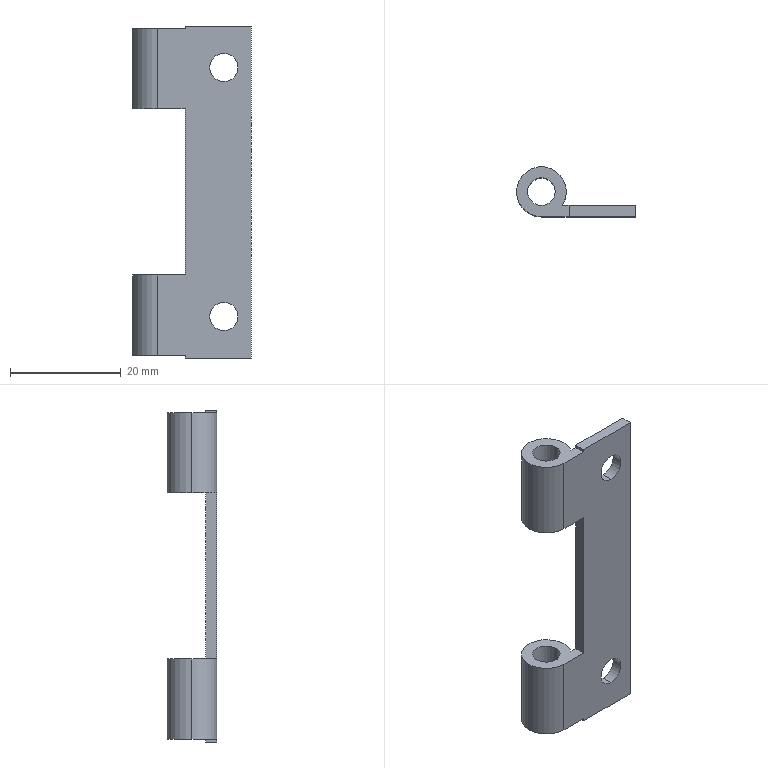Part | STEP file | HI_HFG87-17-001(2)^HFG87-17(2)_Lower机架DoorPlate 2 | 1 solid | 26 faces | box 21.5 x 9 x 60 mm | volume 2771 mm3 | cylinder 14 | plane 12 | commonest cylinder face diameters 9 x6 5 x4 5.1 x4